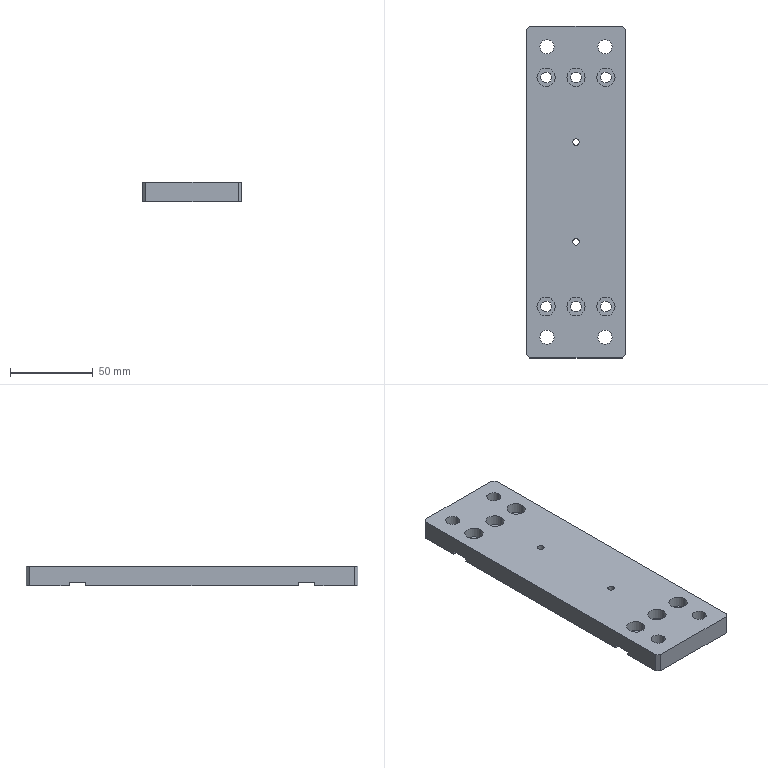Part | SolidWorks | features Cut 2, Chamfer 1, Extrusion 1, HoleWzd 1, ICE 1 | 1 solid | 60 faces | box 60 x 200 x 12 mm | volume 134076 mm3 | cylinder 36 | plane 24 | commonest cylinder face diameters 6.5 x12 11 x12 8.5 x8 4 x4